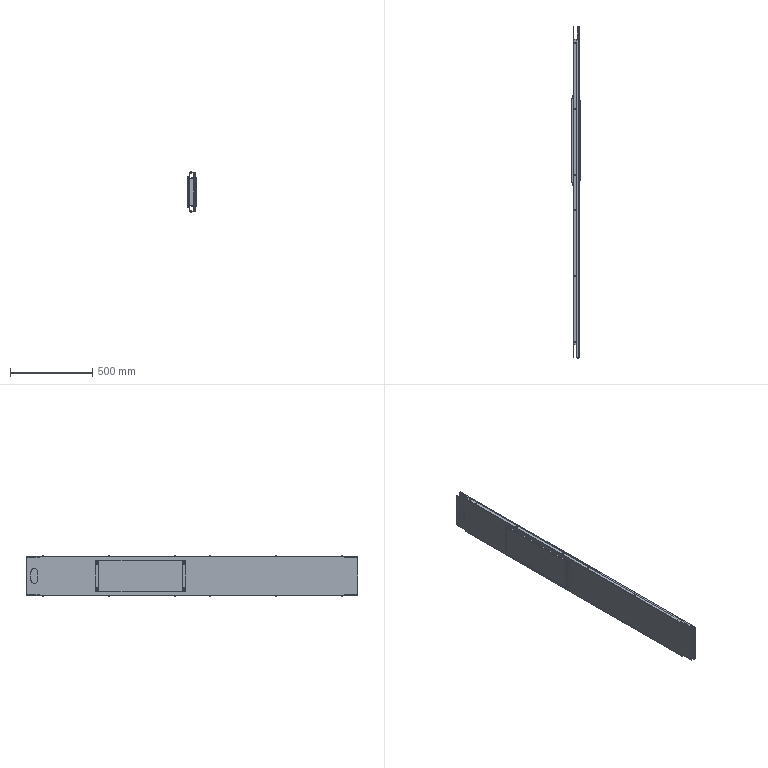Part | 21 solids | 514 faces | box 55 x 2016 x 253 mm | volume 5752629 mm3 | plane 302 | cylinder 212 | commonest cylinder face diameters 7 x39 6 x32 6.2 x24 8 x24 8.2 x24 12 x24